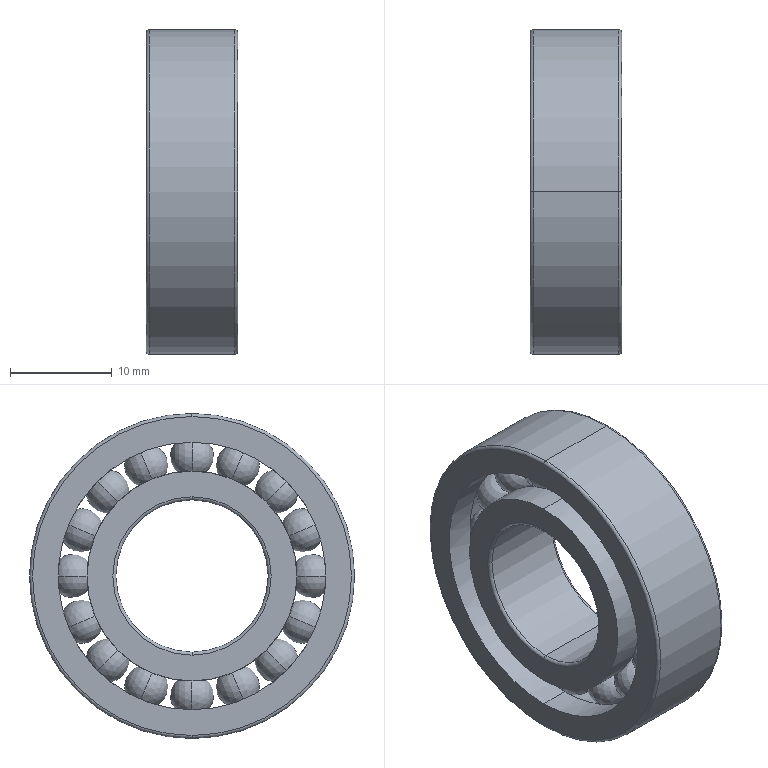Part | STEP file | deep groove ball bearings gb._Rolling bearings 6002 GB 276-94 | 1 solid | 104 faces | box 9 x 32 x 32 mm | volume 4178 mm3 | torus 56 | sphere 32 | cylinder 12 | plane 4 | commonest cylinder face diameters 20.667 x4 26.333 x4 15 x2 32 x2